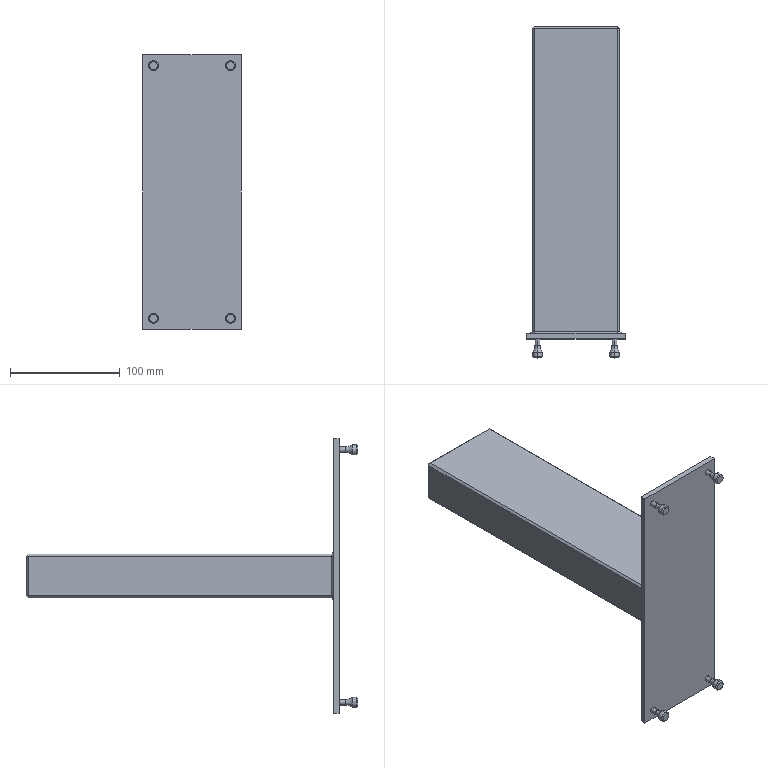Part | SolidWorks | features Chamfer 3, ICE 3, Extrusion 1, Fillet 1 | 1 solid | 65 faces | box 90 x 302 x 250 mm | volume 1008756 mm3 | plane 33 | cone 16 | torus 8 | cylinder 8 | commonest cylinder face diameters 5 x8